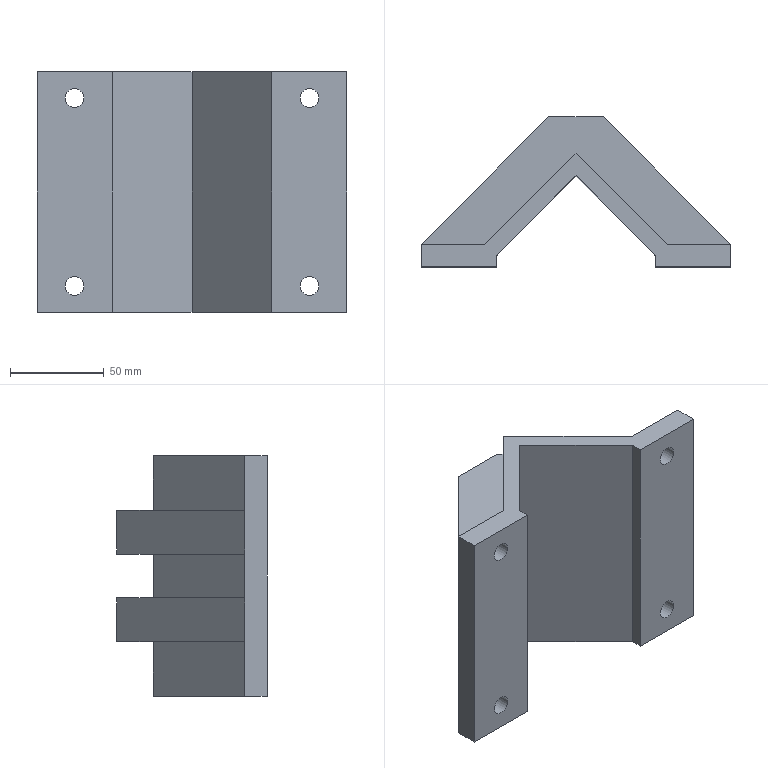Part | STEP file | Y2_DJ_80.step 2 | 1 solid | 36 faces | box 165 x 80 x 128 mm | volume 452320 mm3 | plane 32 | cylinder 4 | commonest cylinder face diameters 10 x4